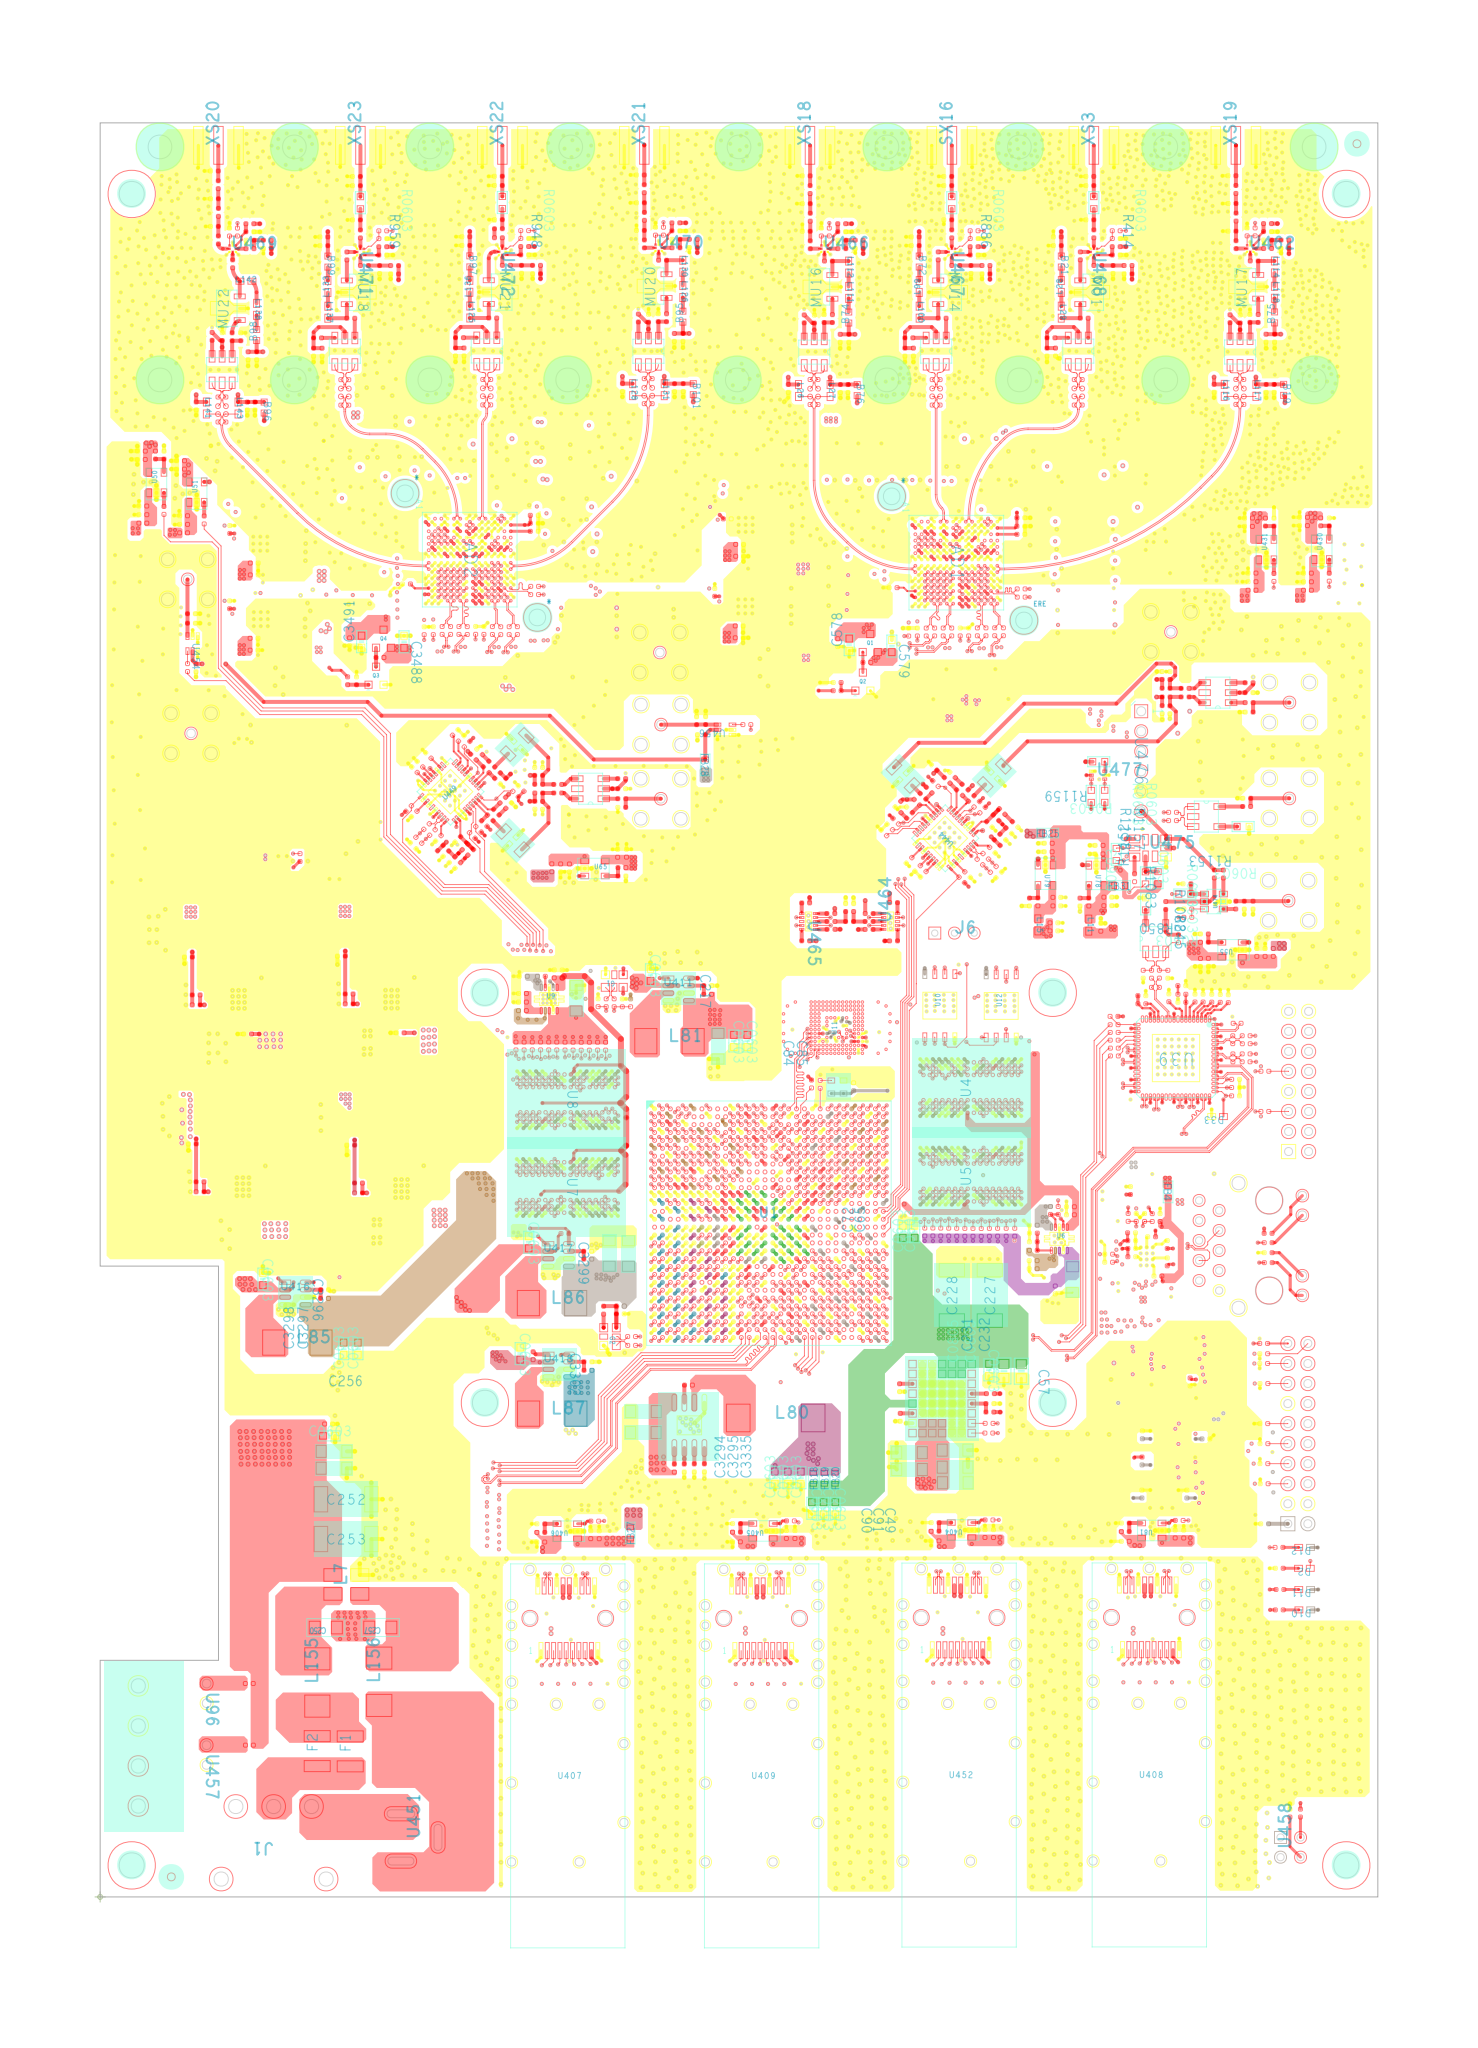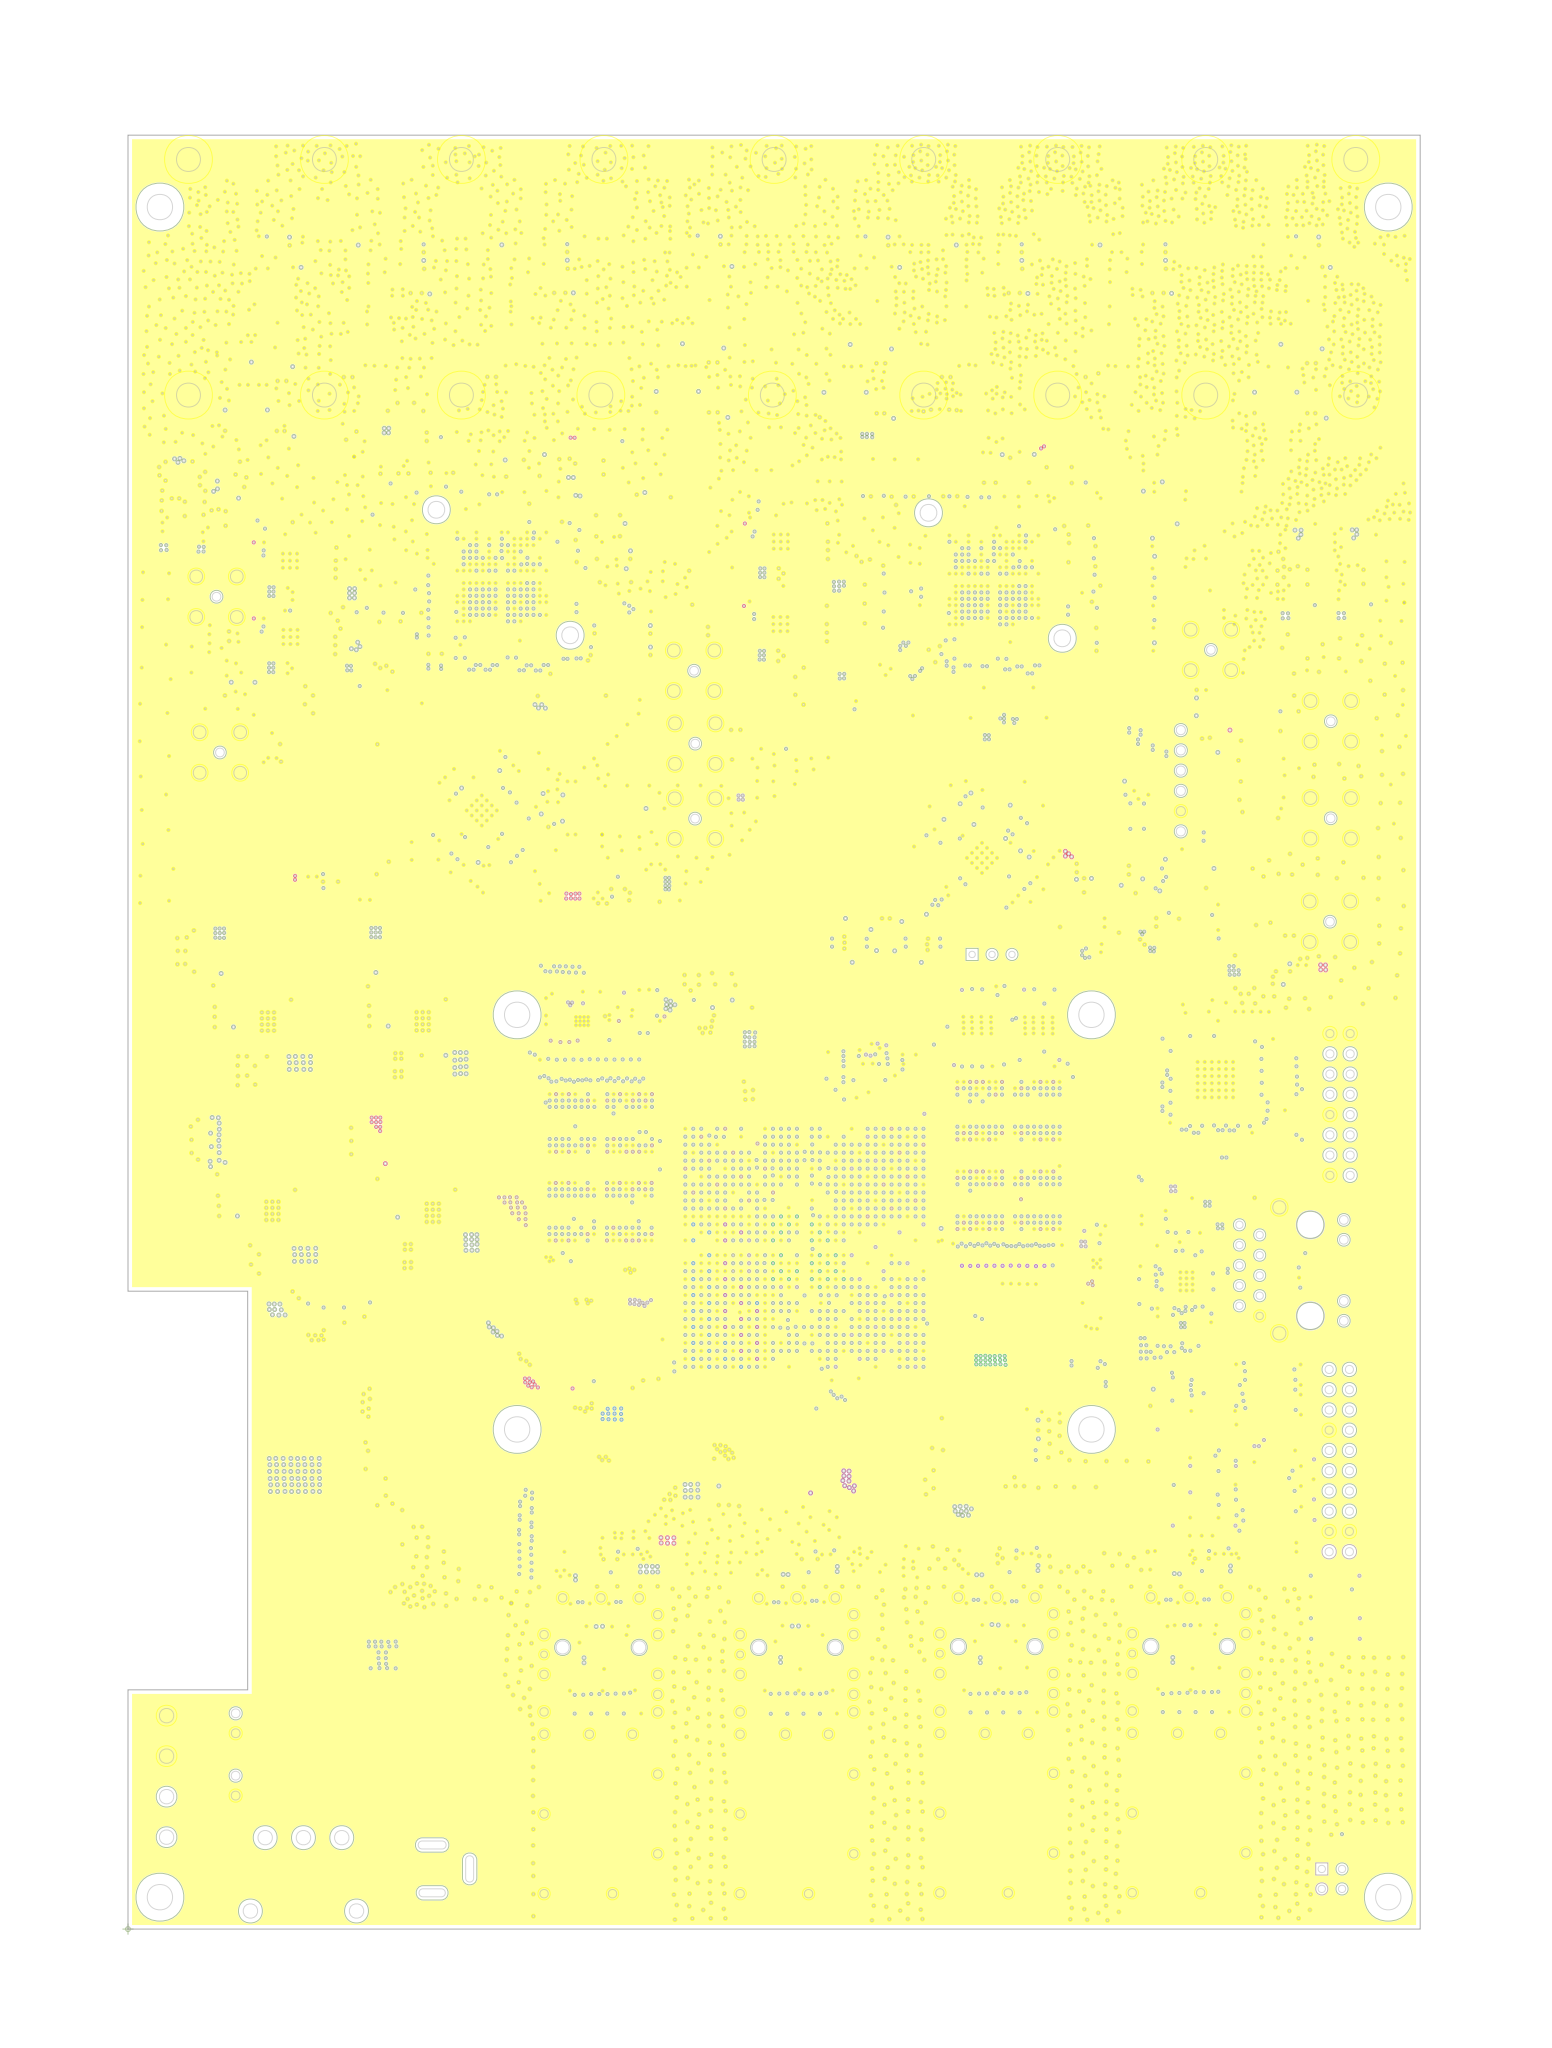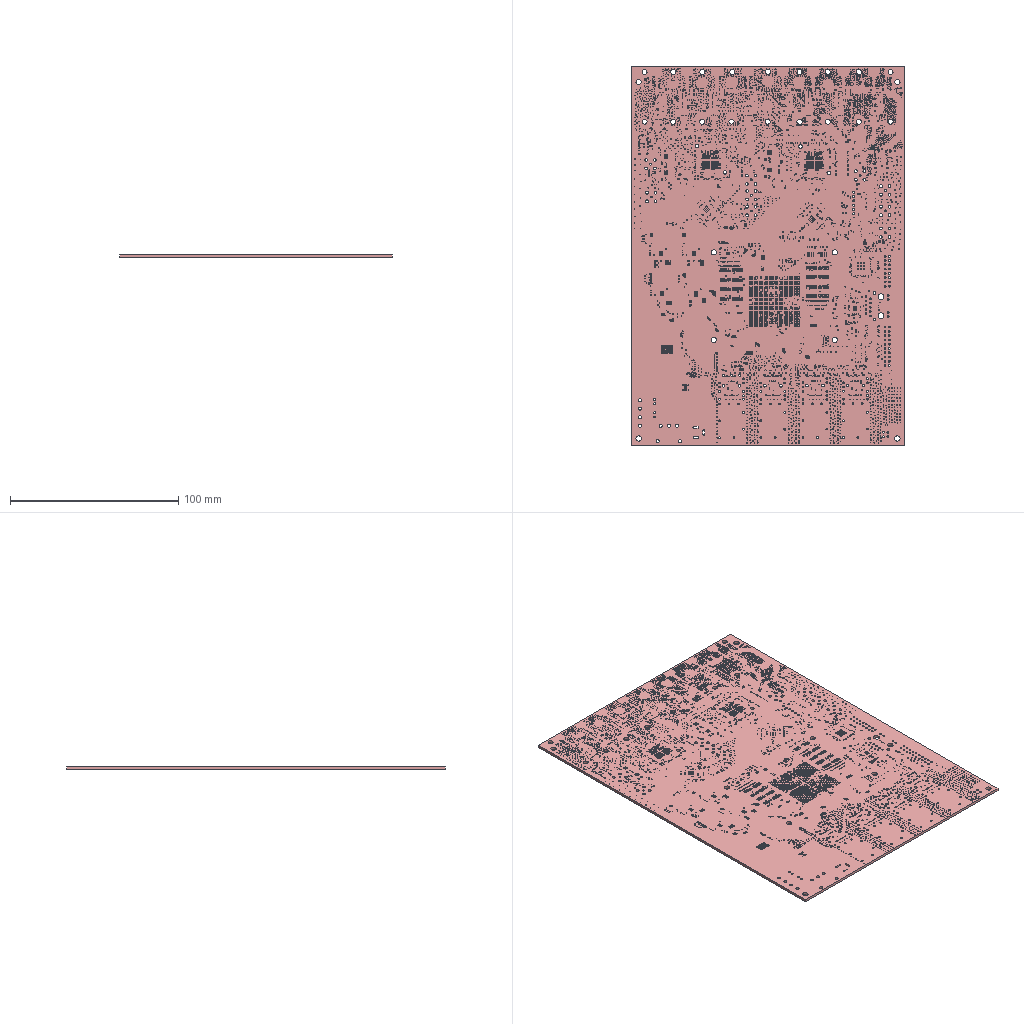Circuit board layout | Cadence Allegro | box 162 x 225 x 1.6 mm
Layer stack:
# Cadence Allegro layer stack of  (unit mm; from the constraint file cross-section; dielectric type: 0 not recorded (Allegro does not mark core vs prepreg), 3 surface material)
index,name,kind,layer,copper_thickness_mm,dielectric_type,dielectric_thickness_mm,dielectric_material,dielectric_constant
0,Top Surface,other,,,,,,
1,TOP,copper,TOP,0.0305,,,,
2,Dielectric1,dielectric,,,0,0.2032,FR-4,4.5
3,GND2,copper,GND2,0.0305,,,,
4,Dielectric2,dielectric,,,0,0.2032,FR-4,4.5
5,SIG3,copper,SIG3,0.0305,,,,
6,Dielectric3,dielectric,,,0,0.2032,FR-4,4.5
7,POWER4,copper,POWER4,0.0305,,,,
8,Dielectric4,dielectric,,,0,0.2032,FR-4,4.5
9,GND5,copper,GND5,0.0305,,,,
10,Dielectric5,dielectric,,,0,0.2032,FR-4,4.5
11,SIG6,copper,SIG6,0.0305,,,,
12,Dielectric6,dielectric,,,0,0.2032,FR-4,4.5
13,POWER7,copper,POWER7,0.0305,,,,
14,Dielectric7,dielectric,,,0,0.2032,FR-4,4.5
15,BOTTOM,copper,BOTTOM,0.0305,,,,
16,Bottom Surface,other,,,,,,
# drill layer pairs: low layer,high layer
drill_pair,TOP,BOTTOM
Part placement, first 543 of 1794 lines:
REFDES,COMP_VALUE,SYM_NAME,SYM_X,SYM_Y,SYM_ROTATE,SYM_MIRROR
25MHZ1,SIT8208AI-2F-33E-25M,3225,5208.251,3540.558,180.000,YES
AD1,AD9371,BGA196,4273.797,6662.298,270.000,NO
AD2,AD9371,BGA196,1844.787,6677.270,270.000,NO
B1,B0603(120R)2A,B0603,4405.607,5888.987,270.000,YES
B2,B0603(120R)2A,B0603,4286.605,5888.999,270.000,YES
B3,B0603(120R)2A,B0603,4053.238,7257.773,90.000,YES
B4,B0603(120R)2A,B0603,3729.200,7257.600,90.000,YES
B5,B0603(120R)2A,B0603,3837.838,7257.117,90.000,YES
B6,B0603(120R)2A,B0603,4156.250,7258.397,90.000,YES
B7,B0603(120R)2A,B0603,3549.608,6505.395,180.000,YES
B8,B0603(120R)2A,B0603,3953.432,7258.123,90.000,YES
B9,B0603(120R)2A,B0603,4976.588,6463.405,0.000,YES
B10,B0603(120R)2A,B0603,3627.097,7257.416,90.000,YES
B11,B0603(120R)2A,B0603,4976.178,6574.105,0.000,YES
B12,B0603(120R)2A,B0603,4975.364,6769.187,0.000,YES
B13,B0603(120R)2A,B0603,3548.000,6409.303,180.000,YES
B14,B0603(120R)2A,B0603,4975.658,6672.293,0.000,YES
B15,B0603(120R)2A,B0603,4973.932,6868.378,0.000,YES
B16,B0603(120R)2A,B0603,3548.890,6693.191,180.000,YES
B17,B0603(120R)2A,B0603,4973.648,6351.366,0.000,YES
B18,B0603(120R)2A,B0603,3549.400,6600.097,180.000,YES
B19,B0603(120R)2A,B0603,5907.800,7552.668,270.000,NO
B21,B0603(120R)2A,B0603,4798.017,8193.507,270.000,NO
B72,B0603(120R)2A,B0603,4088.717,8193.407,270.000,NO
B73,B0603(120R)2A,B0603,5104.886,7024.718,90.000,YES
B74,B0603(120R)2A,B0603,3736.793,7858.695,90.000,NO
B75,B0603(120R)2A,B0603,5862.293,7859.295,90.000,NO
B76,B0603(120R)2A,B0603,3778.842,7551.451,270.000,NO
B77,B0603(120R)2A,B0603,2406.400,6690.500,0.000,YES
B78,B0603(120R)2A,B0603,1100.305,6352.178,270.000,YES
B79,B0603(120R)2A,B0603,2150.138,6006.840,270.000,YES
B80,B0603(120R)2A,B0603,2231.480,6007.048,270.000,YES
B81,B0603(120R)2A,B0603,1283.700,6346.000,270.000,YES
B82,B0603(120R)2A,B0603,2181.100,7127.500,90.000,YES
B83,B0603(120R)2A,B0603,1533.468,7278.589,90.000,YES
B84,B0603(120R)2A,B0603,1178.300,6345.600,270.000,YES
B85,B0603(120R)2A,B0603,1386.571,6345.910,270.000,YES
B86,B0603(120R)2A,B0603,2401.100,6805.800,0.000,YES
B87,B0603(120R)2A,B0603,1644.374,7278.607,90.000,YES
B88,B0603(120R)2A,B0603,1206.300,7281.300,90.000,YES
B89,B0603(120R)2A,B0603,1488.743,7444.574,180.000,YES
B90,B0603(120R)2A,B0603,2400.700,6916.800,0.000,YES
B91,B0603(120R)2A,B0603,1295.385,7280.764,90.000,YES
B92,B0603(120R)2A,B0603,1424.368,7281.109,90.000,YES
B93,B0603(120R)2A,B0603,2476.246,6330.290,0.000,YES
B94,B0603(120R)2A,B0603,2477.386,6437.099,0.000,YES
B95,B0603(120R)2A,B0603,2908.893,7862.995,90.000,NO
B96,B0603(120R)2A,B0603,818.800,7464.268,270.000,NO
B97,B0603(120R)2A,B0603,1845.317,8194.207,270.000,NO
B98,B0603(120R)2A,B0603,781.093,7771.395,90.000,NO
B99,B0603(120R)2A,B0603,1136.817,8193.107,270.000,NO
B100,B0603(120R)2A,B0603,2550.897,6957.122,90.000,YES
B101,B0603(120R)2A,B0603,2960.742,7556.351,270.000,NO
C1,22uF/16V,C0603,3830.654,3338.762,0.000,YES
C2,0.47uF,C0402,3282.110,3399.885,270.000,YES
C3,0.1uF,C0402,3319.624,3399.885,270.000,YES
C4,100uF/6.3V,1206,2541.152,3213.020,90.000,NO
C5,0.47uF,C0402,3552.930,3352.808,180.000,YES
C6,4.7uF,C0402,3672.856,2970.154,270.000,YES
C7,0.1uF,C0402,3761.203,4045.350,270.000,NO
C8,22uF/16V,C0603,3593.157,3287.950,180.000,YES
C9,4.7uF,C0402,3165.053,3246.958,90.000,YES
C10,0.47uF,C0402,3163.712,3129.783,270.000,YES
C11,0.01uF,C0402,3496.001,3698.018,0.000,YES
C13,100uF/6.3V,1206,3084.090,4247.774,270.000,NO
C14,4.7uF,C0402,3434.721,2932.735,90.000,YES
C15,100uF/6.3V,1206,2637.229,3212.797,90.000,NO
C16,4.7uF,C0402,3662.263,3208.192,0.000,YES
C17,100uF/6.3V,1206,3998.258,3294.295,180.000,YES
C18,4.7uF,C0402,3457.064,3151.027,180.000,YES
C19,22uF/16V,C0603,3857.096,2732.465,0.000,YES
C20,4.7uF,C0402,3204.304,3130.532,270.000,YES
C21,22uF/16V,C0603,3712.710,3338.714,180.000,YES
C22,4.7uF,C0402,3028.701,3310.203,180.000,YES
C23,47uF/6.3V,C0603,4255.087,3640.246,0.000,YES
C24,4.7uF,C0402,2989.202,3932.223,0.000,YES
C25,0.47uF,C0402,2948.688,3855.397,180.000,YES
C26,0.01uF,C0402,2830.121,3895.228,0.000,YES
C27,47uF/6.3V,C0603,2643.043,3404.908,90.000,YES
C28,4.7uF,C0402,3202.685,3676.385,90.000,YES
C29,0.47uF,C0402,2191.798,4156.921,0.000,YES
C30,0.01uF,C0402,3085.530,3674.468,90.000,YES
C31,22uF/16V,C0603,3343.337,3904.685,90.000,YES
C32,4.7uF,C0402,3263.279,3695.778,180.000,YES
C33,0.47uF,C0402,3279.240,3836.426,90.000,YES
C34,22uF/16V,C0603,3265.198,3618.237,90.000,YES
C35,4.7uF,C0402,2868.948,3695.869,180.000,YES
C36,0.47uF,C0402,2135.492,3808.029,0.000,YES
C37,22uF/16V,C0603,2274.439,4014.844,180.000,YES
C38,4.7uF,C0402,3790.230,3596.228,90.000,YES
C39,4.7uF,C0402,2828.124,3934.694,0.000,YES
C40,0.47uF,C0402,4571.400,3789.205,90.000,YES
C41,0.47uF,C0402,3086.326,3915.123,180.000,YES
C42,0.47uF,C0402,2098.651,4153.939,180.000,YES
C43,0.47uF,C0402,2989.760,3976.398,0.000,YES
C44,0.47uF,C0402,3163.865,3719.834,270.000,YES
C45,0.47uF,C0402,2337.208,4084.462,270.000,YES
C46,0.01uF,C0402,3593.915,3556.411,90.000,YES
C47,0.01uF,C0402,3692.397,3577.574,0.000,YES
C49,22uF/16V,C0603,3669.926,1940.763,270.000,NO
C50,4.7uF,C0402,3283.598,3284.397,90.000,YES
C51,4.7uF,C0402,3456.957,3269.693,0.000,YES
C52,4.7uF,C0402,3240.206,3286.367,90.000,YES
C53,0.47uF,C0402,3375.202,3152.212,180.000,YES
C54,0.47uF,C0402,3375.775,3191.175,0.000,YES
C55,0.47uF,C0402,3376.301,3233.318,180.000,YES
C56,0.47uF,C0402,3516.162,3212.572,90.000,YES
C57,22uF/16V,C0603,4436.429,2631.932,270.000,NO
C58,4.7uF,C0402,3377.369,3269.745,0.000,YES
C59,4.7uF,C0402,3203.118,3291.095,90.000,YES
C60,4.7uF,C0402,3455.204,3307.943,180.000,YES
C61,0.47uF,C0402,3378.599,3499.208,0.000,YES
C62,0.47uF,C0402,3454.840,3191.970,0.000,YES
C63,0.47uF,C0402,3282.911,3205.983,270.000,YES
C64,0.47uF,C0402,3319.899,3284.661,90.000,YES
C65,22uF/16V,C0603,4066.127,3321.362,90.000,NO
C66,4.7uF,C0402,3375.555,3308.285,180.000,YES
C68,4.7uF,C0402,3164.578,3331.561,270.000,YES
C69,0.47uF,C0402,3240.019,3209.113,270.000,YES
C70,0.47uF,C0402,3243.634,3346.078,0.000,YES
C71,0.47uF,C0402,3203.221,3210.589,90.000,YES
C72,22uF/16V,C0603,4006.967,3320.968,90.000,NO
C73,4.7uF,C0402,3324.988,3520.620,270.000,YES
C74,4.7uF,C0402,3298.114,3463.355,0.000,YES
C75,4.7uF,C0402,3455.381,3379.091,0.000,YES
C76,0.47uF,C0402,3319.238,3205.510,90.000,YES
C77,0.47uF,C0402,3456.495,3231.055,180.000,YES
C78,0.47uF,C0402,3455.189,3345.503,0.000,YES
C79,0.47uF,C0402,3180.481,3461.948,180.000,YES
C80,4.7uF,C0402,3397.536,3400.117,270.000,YES
C81,4.7uF,C0402,3376.975,3464.247,0.000,YES
C82,0.47uF,C0402,3204.432,3400.226,270.000,YES
C83,22uF/16V,C0603,3596.108,3400.652,180.000,YES
C84,22uF/16V,C0603,3163.245,4274.157,270.000,NO
C85,22uF/16V,C0603,3229.807,4273.998,270.000,NO
C86,0.47uF,C0402,3457.062,3498.105,0.000,YES
C87,10uF/10V,C0402,3456.367,3462.528,0.000,YES
C88,22uF/16V,C0603,3329.971,3621.638,270.000,YES
C89,22uF/16V,C0603,3417.758,3592.051,270.000,YES
C90,22uF/16V,C0603,3552.655,1940.553,270.000,NO
C91,22uF/16V,C0603,3611.308,1940.553,270.000,NO
C94,4.7uF,C0402,2947.900,2954.838,0.000,YES
C95,4.7uF,C0402,3003.855,3442.776,90.000,YES
C96,0.47uF,C0402,2945.464,3462.637,180.000,YES
C97,0.47uF,C0402,2928.668,3205.993,270.000,YES
C98,0.47uF,C0402,2944.326,3067.849,180.000,YES
C99,0.47uF,C0402,2929.729,3286.593,90.000,YES
C100,4.7uF,C0402,2769.759,3440.933,270.000,YES
C101,4.7uF,C0402,2808.916,3400.458,90.000,YES
C102,0.47uF,C0402,2866.890,3344.611,180.000,YES
C103,0.47uF,C0402,2770.842,3288.582,270.000,YES
C104,0.47uF,C0402,2770.346,3208.484,270.000,YES
C105,0.47uF,C0402,2866.150,3265.631,180.000,YES
C107,4.7uF,C0402,2957.003,3359.219,180.000,YES
C108,0.47uF,C0402,3025.398,3268.001,0.000,YES
C109,0.01uF,C0402,4452.964,3603.929,0.000,YES
C110,0.01uF,C0402,4452.910,3645.066,180.000,YES
C111,0.01uF,C0402,4512.400,4218.412,180.000,YES
C112,0.01uF,C0402,4512.326,4257.048,0.000,YES
C114,4.7uF,C0402,4157.093,3230.017,270.000,YES
C115,4.7uF,C0402,4116.148,3230.147,270.000,YES
C116,4.7uF,C0402,4276.477,3230.017,270.000,YES
C117,1uF,C0402,4195.753,3229.753,270.000,YES
C118,1uF,C0402,4316.713,3230.017,270.000,YES
C119,1uF,C0402,4236.399,3229.753,270.000,YES
C120,1uF,C0402,4356.965,3230.017,270.000,YES
C121,0.1uF,C0402,4398.458,3230.147,270.000,YES
C122,0.1uF,C0402,4438.840,3230.079,270.000,YES
C123,0.1uF,C0402,4523.188,3230.016,270.000,YES
C124,0.1uF,C0402,4481.455,3230.146,270.000,YES
C125,4.7uF,C0402,4308.410,3768.213,180.000,YES
C132,0.1uF,C0402,4060.502,3489.044,90.000,YES
C133,0.1uF,C0402,4219.623,3769.040,0.000,YES
C134,0.1uF,C0402,4496.172,3791.569,90.000,YES
C135,0.1uF,C0402,4129.276,3768.560,180.000,YES
C136,0.1uF,C0402,4219.313,3549.633,0.000,YES
C137,4.7uF,C0402,4137.020,4211.808,180.000,YES
C138,0.1uF,C0402,4482.343,3865.702,180.000,YES
C139,0.1uF,C0402,4321.272,4214.028,180.000,YES
C140,0.1uF,C0402,4268.090,3870.491,0.000,YES
C141,0.1uF,C0402,4229.989,4213.107,0.000,YES
C142,0.1uF,C0402,4064.019,4138.470,90.000,YES
C143,0.01uF,C0402,4658.410,3314.351,0.000,NO
C144,4.7uF,C0402,4657.886,3353.910,0.000,NO
C145,0.1uF,C0402,4843.347,3406.119,0.000,NO
C146,100uF/6.3V,1206,4854.765,3082.881,270.000,NO
C147,10uF/10V,C0402,4657.323,3136.541,0.000,NO
C148,10uF/10V,C0402,4657.323,3177.093,0.000,NO
C149,10uF/10V,C0402,4767.768,3030.771,90.000,NO
C150,4.7uF,C0402,4782.105,3427.837,90.000,YES
C151,4.7uF,C0402,4843.347,3446.135,0.000,NO
C152,4.7uF,C0402,2370.016,3373.031,0.000,YES
C153,0.1uF,C0402,2574.421,3709.999,180.000,YES
C154,0.1uF,C0402,2398.043,3709.023,180.000,YES
C155,0.1uF,C0402,2486.232,3709.905,180.000,YES
C156,0.1uF,C0402,2458.803,3372.204,180.000,YES
C157,0.1uF,C0402,2559.985,4151.524,180.000,YES
C158,4.7uF,C0402,2549.280,3808.934,0.000,YES
C159,0.1uF,C0402,2467.465,4149.855,180.000,YES
C160,0.1uF,C0402,2554.213,4029.986,180.000,YES
C161,0.1uF,C0402,2549.150,3372.684,0.000,YES
C162,0.1uF,C0402,2456.312,3807.634,180.000,YES
C163,0.1uF,C0402,2365.028,3806.713,0.000,YES
C164,4.7uF,C0402,2359.807,4336.390,90.000,YES
C165,4.7uF,C0402,2074.127,4336.260,90.000,YES
C166,4.7uF,C0402,2481.948,4336.390,90.000,YES
C167,1uF,C0402,2278.925,4335.996,90.000,YES
C168,1uF,C0402,2441.712,4336.654,90.000,YES
C169,1uF,C0402,2319.177,4336.390,90.000,YES
C170,1uF,C0402,2401.066,4336.654,90.000,YES
C171,0.1uF,C0402,2115.461,4335.997,90.000,YES
C172,0.1uF,C0402,2157.192,4335.473,90.000,YES
C173,0.1uF,C0402,2198.625,4335.540,90.000,YES
C174,0.1uF,C0402,2238.614,4335.867,90.000,YES
C175,0.01uF,C0402,2238.134,3487.898,180.000,YES
C176,0.01uF,C0402,2187.696,3935.500,0.000,YES
C177,0.01uF,C0402,2317.112,3684.265,180.000,YES
C178,0.01uF,C0402,2380.424,4148.526,0.000,YES
C179,4.7uF,C0402,2112.164,4597.106,0.000,NO
C180,0.01uF,C0402,2108.013,4511.201,0.000,NO
C181,100uF/6.3V,1206,2376.054,4487.863,90.000,NO
C182,10uF/10V,C0402,2375.648,4445.049,90.000,YES
C183,10uF/10V,C0402,2202.599,4425.134,180.000,YES
C184,10uF/10V,C0402,2293.544,4425.134,0.000,YES
C185,4.7uF,C0402,2281.040,4541.705,0.000,YES
C186,0.1uF,C0402,2306.663,4608.586,270.000,NO
C187,4.7uF,C0402,2266.661,4608.980,270.000,NO
C188,0.1uF,C0402,4137.075,4606.477,0.000,YES
C189,0.1uF,C0402,4442.457,4606.083,0.000,YES
C190,10uF/10V,C0402,3680.505,4151.682,270.000,YES
C191,1uF,C0402,3595.721,4149.056,270.000,YES
C192,0.1uF,C0402,3667.390,4295.548,0.000,YES
C193,10uF/10V,C0402,3798.285,4351.080,0.000,YES
C194,0.1uF,C0402,3780.110,4289.215,270.000,YES
C195,0.1uF,C0402,3666.997,4246.036,0.000,YES
C196,10uF/10V,C0402,3869.359,4242.142,0.000,YES
C197,0.1uF,C0402,3868.835,4292.493,0.000,YES
C198,0.1uF,C0402,3588.556,4291.839,270.000,YES
C199,0.1uF,C0402,3868.835,4198.099,0.000,YES
C200,0.1uF,C0402,2489.044,4580.813,270.000,YES
C201,4.7uF,C0402,2448.178,4580.813,270.000,YES
C202,0.1uF,C0402,2572.059,4580.345,90.000,YES
C203,0.1uF,C0402,2565.664,4464.674,90.000,NO
C204,0.1uF,C0402,2525.900,4464.804,90.000,NO
C205,0.1uF,C0402,2596.400,2911.400,180.000,NO
C206,0.1uF,C0402,3908.531,3207.189,90.000,YES
C207,4.7uF,C0402,3770.989,3233.304,0.000,YES
C208,0.1uF,C0402,2652.855,2797.985,180.000,NO
C209,0.1uF,C0402,2653.119,2753.889,180.000,NO
C210,0.1uF,C0402,3369.153,2103.770,270.000,YES
C211,150pF,C0402,2965.825,2142.235,90.000,YES
C212,2.2uF,C0402,2965.683,2142.131,90.000,NO
C213,10nF,C0402,3016.162,2142.458,90.000,NO
C214,22uF/25V,1206,2711.969,2423.426,0.000,NO
C217,22uF/10V,C0603,2747.145,4604.273,270.000,NO
C219,22uF,C0603,3160.760,4285.788,270.000,YES
C220,22uF,C0603,3084.855,4281.854,270.000,YES
C222,22uF/25V,1206,4040.186,2134.004,0.000,NO
C223,22uF/25V,1206,4268.676,2068.106,180.000,NO
C224,22uF/25V,1206,4040.166,2218.238,0.000,NO
C225,22uF/25V,1206,4267.686,2145.845,180.000,NO
C226,22uF/25V,1206,4267.492,2230.949,180.000,NO
C227,470uF,C7343,4441.112,3003.981,90.000,NO
C228,470uF,C7343,4251.594,3004.145,90.000,NO
C229,47uF,C0805,4511.368,2626.963,270.000,YES
C230,47uF,C0805,4598.202,2626.669,270.000,YES
C231,47uF,C0805,4511.408,2626.375,90.000,NO
C232,47uF,C0805,4598.242,2624.899,90.000,NO
C250,1000pF/1KV,C1206,1126.316,1344.967,180.000,NO
C252,100uF/25V,C7343,1228.043,1985.644,0.000,NO
C253,100uF/25V,C7343,1228.043,1787.054,0.000,NO
C254,22uF/25V,1206,1167.429,2224.818,180.000,NO
C255,22uF/25V,1206,1167.203,2140.482,180.000,NO
C256,4.7uF/25V,C0603,1142.948,2302.052,0.000,NO
C257,1000pF/1KV,C1206,1398.311,1345.391,180.000,NO
C258,0.01uF/25V,C0402,1140.200,2361.400,180.000,NO
C259,1000pF/1KV,C1206,1397.614,1344.475,180.000,YES
C352,100pF,C0402,712.695,5809.871,0.000,YES
C355,1nF,C0402,1380.447,5303.903,0.000,YES
C356,10uF,C0402,1380.321,5343.891,180.000,YES
C365,22uF,C0603,5220.442,1234.619,180.000,YES
C366,0.1uF,C0402,5272.193,1535.570,0.000,YES
C367,22uF,C0603,5300.955,1457.558,180.000,YES
C368,0.1uF,C0402,5185.513,1535.964,180.000,YES
C380,100nF,C0402,5248.691,3296.316,180.000,NO
C381,100nF,C0402,5326.829,3257.485,90.000,NO
C382,100nF,C0402,5326.829,3170.988,90.000,NO
C383,100nF,C0402,5035.416,3374.722,180.000,YES
C384,2.2uF,C0402,5050.675,3480.546,180.000,YES
C385,100nF,C0402,5050.171,3522.732,0.000,YES
C386,4.7uF,C0402,5149.757,3196.646,180.000,NO
C387,100nF,C0402,5149.648,3237.870,0.000,NO
C388,4.7uF,C0402,5148.404,3315.946,180.000,NO
C389,100nF,C0402,5149.061,3276.876,0.000,NO
C390,100nF,C0402,5290.779,3392.428,90.000,NO
C391,100nF,C0402,5280.112,3100.104,180.000,NO
C392,4.7uF,C0402,5101.730,3047.601,180.000,YES
C393,100nF,C0402,5102.136,3005.842,0.000,YES
C394,100nF,C0402,5505.168,3611.138,0.000,YES
C395,2.2uF,C0402,5303.502,2996.149,0.000,YES
C396,100nF,C0402,5142.921,3527.040,90.000,NO
C397,100nF,C0402,5251.981,3391.948,90.000,YES
C398,0.01uF,C0402,5812.761,1863.074,180.000,NO
C399,10uF,C0402,5812.349,1862.970,0.000,YES
C400,100nF,C0402,5095.861,2583.653,180.000,YES
C401,100nF,C0402,5440.963,2571.317,90.000,NO
C402,1uF,C0402,5627.791,4375.463,90.000,YES
C403,0.01uF,C0402,5175.584,4317.224,270.000,YES
C404,1uF,C0402,4995.073,4841.746,270.000,NO
C405,0.01uF,C0402,5243.352,4363.505,270.000,YES
C410,0.01uF,C0402,5361.158,4364.476,270.000,YES
C414,0.01uF,C0402,5518.485,4383.892,180.000,YES
C418,1uF,C0402,4760.990,4863.912,180.000,NO
C419,0.01uF,C0402,5194.707,4139.989,0.000,YES
C422,0.01uF,C0402,5194.918,4198.301,0.000,YES
C426,0.01uF,C0402,5241.692,4013.250,90.000,YES
C427,1uF,C0402,5399.376,4550.038,0.000,NO
C428,180pF,C0402,5399.770,4467.298,180.000,NO
C430,0.01uF,C0402,5301.974,4013.067,90.000,YES
C432,0.01uF,C0402,5361.074,4013.672,90.000,YES
C434,0.01uF,C0402,5420.174,4013.095,90.000,YES
C435,0.1uF,C0402,5334.794,4489.495,90.000,NO
C436,0.1uF,C0402,5248.494,4607.264,90.000,NO
C437,0.1uF,C0402,5287.500,4607.447,90.000,NO
C439,0.01uF,C0402,5478.880,4013.700,90.000,YES
C440,1nF,C0402,5200.129,4459.635,180.000,NO
C441,470nF,C0402,5199.884,4500.223,0.000,NO
C445,0.1uF,C0402,4421.656,6316.956,270.000,NO
C446,1uF,C0402,4074.985,6823.065,180.000,YES
C447,0.1uF,C0402,4378.999,6316.810,270.000,NO
C448,100uF,1206,4469.629,6019.758,0.000,YES
C449,1uF,C0402,4426.940,6085.104,0.000,YES
C450,1uF,C0402,4398.099,6981.916,90.000,YES
C451,1uF,C0402,3748.918,7147.533,0.000,YES
C452,0.01uF,C0402,3749.346,7103.567,0.000,YES
C453,0.1uF,C0402,4508.732,6317.218,270.000,NO
C454,0.1uF,C0402,4421.968,6317.137,90.000,YES
C455,1uF,C0402,3958.405,6537.435,0.000,NO
C456,0.1uF,C0402,4378.995,6316.772,90.000,YES
C457,0.1uF,C0402,4508.779,6317.293,90.000,YES
C458,1uF,C0402,4597.321,6749.600,0.000,YES
C459,1uF,C0402,3858.064,7151.264,0.000,YES
C460,100uF,1206,4222.981,6024.986,180.000,YES
C461,0.1uF,C0402,4465.240,6317.223,90.000,YES
C462,1uF,C0402,4268.513,6130.064,180.000,YES
C463,0.01uF,C0402,4268.358,6087.164,180.000,YES
C464,0.1uF,C0402,4250.703,6316.251,270.000,NO
C465,0.1uF,C0402,4208.409,6316.256,270.000,NO
C466,0.1uF,C0402,4165.418,6316.201,270.000,NO
C467,0.1uF,C0402,4250.446,6316.092,90.000,YES
C468,0.1uF,C0402,4208.435,6316.426,90.000,YES
C469,1uF,C0402,4277.325,6595.195,90.000,YES
C470,0.01uF,C0402,4277.599,6508.325,270.000,YES
C471,0.1uF,C0402,4165.375,6316.269,90.000,YES
C472,0.1uF,C0402,4123.997,6316.204,90.000,YES
C473,0.01uF,C0402,4426.968,6130.368,0.000,YES
C474,0.1uF,C0402,4465.401,6317.258,270.000,NO
C475,0.01uF,C0402,3857.973,7105.722,0.000,YES
C476,0.1uF,C0402,4123.569,6316.054,270.000,NO
C477,1uF,C0402,4073.654,7110.654,0.000,YES
C478,0.01uF,C0402,4073.294,7152.974,0.000,YES
C479,1uF,C0402,4175.745,7111.336,0.000,YES
C480,0.01uF,C0402,4175.865,7153.262,0.000,YES
C481,1uF,C0402,3663.125,6525.233,90.000,YES
C482,0.01uF,C0402,3703.545,6525.353,90.000,YES
C483,1uF,C0402,3972.901,7151.976,0.000,YES
C484,0.01uF,C0402,3973.217,7109.586,0.000,YES
C485,1uF,C0402,4865.951,6444.874,270.000,YES
C486,0.01uF,C0402,4822.773,6444.853,270.000,YES
C487,0R,C0402,3958.306,6578.946,180.000,YES
C488,1uF,C0402,3647.363,7100.609,0.000,YES
C489,0.01uF,C0402,3647.503,7143.653,0.000,YES
C490,100uF,1206,3691.089,7032.129,0.000,YES
C491,1uF,C0402,4826.117,6554.678,270.000,YES
C492,0.01uF,C0402,4867.661,6554.932,270.000,YES
C493,0R,C0402,3958.349,6619.526,180.000,YES
C494,1uF,C0402,4865.757,6748.812,270.000,YES
C495,0.01uF,C0402,4823.761,6748.918,270.000,YES
C496,1uF,C0402,3664.289,6428.545,90.000,YES
C497,0.01uF,C0402,3707.073,6428.340,90.000,YES
C498,1uF,C0402,4822.835,6653.437,270.000,YES
C499,0.01uF,C0402,4865.943,6652.826,270.000,YES
C500,10uF,C0402,5028.049,6848.314,270.000,YES
C501,1uF,C0402,4864.753,6849.005,270.000,YES
C502,0.01uF,C0402,4821.459,6848.913,270.000,YES
C503,1uF,C0402,4595.839,6886.418,180.000,NO
C504,1uF,C0402,4595.748,6844.124,180.000,NO
C505,1uF,C0402,3703.093,6713.232,90.000,YES
C506,0.01uF,C0402,3661.561,6713.561,90.000,YES
C507,10uF,C0402,5028.431,6331.915,270.000,YES
C508,0.01uF,C0402,4821.353,6331.673,270.000,YES
C509,1uF,C0402,4864.739,6332.039,270.000,YES
C510,1uF,C0402,3660.747,6619.490,90.000,YES
C511,0.01uF,C0402,3704.713,6619.468,90.000,YES
C512,10uF,C0402,5030.549,6653.290,270.000,YES
C513,10uF,C0402,5027.481,6750.226,270.000,YES
C514,0.01uF,C0402,3576.759,6750.937,0.000,YES
C515,0.01uF,C0402,5030.025,6444.502,270.000,YES
C516,0.01uF,C0402,5030.731,6554.639,270.000,YES
C517,100uF,1206,3963.741,7399.616,90.000,YES
C518,100uF,1206,4053.967,7399.910,90.000,YES
C519,100uF,1206,3398.062,6094.923,180.000,YES
C520,100uF,1206,3398.950,6183.179,180.000,YES
C536,10uF/10V,C0402,5859.872,7532.525,270.000,NO
C537,0.01uF,C0402,5820.636,7532.557,270.000,NO
C538,0.2pF,C0402,3563.626,7451.933,0.000,NO
C539,NC,C0402,3563.583,7576.701,0.000,NO
C540,3pF,C0402,3565.303,7878.416,270.000,NO
C541,43pF,C0402,3565.477,7878.532,270.000,YES
C542,0.01uF,C0402,5560.478,7532.958,270.000,NO
C545,100pF,C0402,4462.885,6982.332,90.000,YES
C546,100pF,C0402,4507.107,6982.543,90.000,YES
C547,NC,C0402,4492.577,7240.028,180.000,YES
C548,NC,C0402,4493.122,7158.656,0.000,YES
C549,100pF,C0402,4306.359,6980.838,90.000,YES
C550,NC,C0402,4334.669,7235.682,180.000,YES
C551,NC,C0402,4334.808,7155.192,0.000,YES
C552,100pF,C0402,4350.881,6981.049,90.000,YES
C563,10uF,C0402,3190.025,6287.518,180.000,YES
C564,1uF,C0402,3189.980,6346.534,180.000,NO
C565,0.1uF,C0402,3190.036,6287.074,180.000,NO
C566,10uF,C0402,3403.362,6443.148,180.000,YES
C567,1uF,C0402,3403.345,6358.548,0.000,YES
C568,0.1uF,C0402,3403.795,6401.748,0.000,YES
C569,1uF,C0402,3067.900,6513.900,270.000,NO
C570,0.01uF,C0402,3253.375,6602.360,180.000,YES
C577,2.2uF,C0402,3951.607,6236.086,90.000,YES
C578,22uF,C0603,3952.003,6245.620,90.000,NO
C579,22uF,C0603,3739.093,6253.088,270.000,NO
C580,2.2uF,C0402,3682.098,6262.853,90.000,NO
C585,10uF/10V,C0402,213.105,6901.866,0.000,NO
C586,0.1uF,C0402,212.988,6945.078,0.000,NO
C587,10uF/10V,C0402,205.681,7219.312,0.000,NO
C588,0.1uF,C0402,205.416,7177.640,0.000,NO
C589,10uF/10V,C0402,416.535,6853.372,0.000,NO
C590,0.1uF,C0402,416.418,6896.584,0.000,NO
C591,10uF/10V,C0402,401.411,7171.018,0.000,NO
C592,0.1uF,C0402,401.146,7129.346,0.000,NO
C593,10uF/10V,C0402,4778.110,8245.468,0.000,NO
C594,0.1uF,C0402,4777.999,8289.140,0.000,NO
C596,220pF,C0402,4892.744,8194.266,270.000,NO
C597,220pF,C0402,4912.362,7883.137,0.000,NO
C598,NC,C0402,4940.419,8374.200,180.000,NO
C622,10uF,C0402,5773.856,4715.958,270.000,NO
C623,0.01uF,C0402,5815.026,4716.051,270.000,NO
C624,10uF,C0402,5531.854,4666.851,90.000,NO
C625,0.01uF,C0402,5492.538,4666.270,90.000,NO
C634,10uF,C0402,2342.467,5138.012,90.000,NO
C635,0.01uF,C0402,2298.697,5138.319,90.000,NO
C636,10uF,C0402,2583.169,5211.019,270.000,NO
C637,0.01uF,C0402,2627.285,5211.500,270.000,NO
C815,4.7uF,C0402,2967.358,3208.973,270.000,YES
C816,4.7uF,C0402,3142.477,3068.295,0.000,YES
C817,0.47uF,C0402,2944.432,3423.159,180.000,YES
C818,0.47uF,C0402,2964.600,3127.776,270.000,YES
C819,0.47uF,C0402,3007.152,3166.055,270.000,YES
C820,0.47uF,C0402,3043.794,3088.892,270.000,YES
C821,4.7uF,C0402,2787.048,2951.147,180.000,YES
C822,4.7uF,C0402,2787.235,3108.812,180.000,YES
C823,0.47uF,C0402,2787.076,2832.159,180.000,YES
C824,0.47uF,C0402,2865.937,2793.153,180.000,YES
C825,0.47uF,C0402,2786.016,3068.559,180.000,YES
C826,0.47uF,C0402,2786.865,2911.353,180.000,YES
C827,4.7uF,C0402,2944.920,2911.353,180.000,YES
C828,4.7uF,C0402,2866.575,2871.953,180.000,YES
C829,0.47uF,C0402,3023.626,2793.547,180.000,YES
C830,0.47uF,C0402,2944.887,2832.947,180.000,YES
C831,0.47uF,C0402,2866.148,2951.541,180.000,YES
C832,0.47uF,C0402,2866.603,3028.765,180.000,YES
C833,4.7uF,C0402,3141.234,2987.919,0.000,YES
C834,4.7uF,C0402,3043.459,3011.263,90.000,YES
C835,0.47uF,C0402,3121.806,2813.153,270.000,YES
C836,0.47uF,C0402,3141.933,2911.877,0.000,YES
C837,0.47uF,C0402,3023.992,2871.559,180.000,YES
C838,0.47uF,C0402,3025.629,2949.965,180.000,YES
C839,0.47uF,C0402,2866.026,3462.559,180.000,YES
C840,0.47uF,C0402,2866.481,3107.959,180.000,YES
C841,0.47uF,C0402,2865.754,3187.547,180.000,YES
C842,0.47uF,C0402,3606.820,2759.325,270.000,YES
C843,0.47uF,C0402,3498.076,2729.442,270.000,YES
C844,0.47uF,C0402,3808.422,3109.001,0.000,YES
C845,0.47uF,C0402,3590.142,2974.284,90.000,YES
C846,0.47uF,C0402,3239.924,3127.758,90.000,YES
C847,0.47uF,C0402,3316.836,2971.602,270.000,YES
C848,0.47uF,C0402,3204.022,2815.319,90.000,YES
C849,0.47uF,C0402,3262.029,2875.893,180.000,YES
C2866,10uF,C0402,4986.025,5208.062,0.000,NO
C2867,0.01uF,C0402,4986.419,5250.614,0.000,NO
C2868,10uF,C0402,5029.961,4992.046,180.000,NO
C2869,0.01uF,C0402,5029.961,4949.494,180.000,NO
C2870,10uF,C0402,4732.295,5218.650,0.000,NO
C2871,0.01uF,C0402,4732.689,5261.202,0.000,NO
C2872,10uF,C0402,4775.653,4991.028,180.000,NO
C2873,0.01uF,C0402,4775.653,4948.476,180.000,NO
C2880,10nF,C0402,4638.917,4967.817,270.000,NO
C2881,10nF,C0402,4890.987,4967.605,270.000,NO
C2882,10uF,C0402,5366.359,1812.158,270.000,NO
C2883,0.1uF,C0402,5408.911,1811.764,270.000,NO
C2884,10uF,C0402,5116.957,1775.516,0.000,NO
C2886,10nF,C0402,5117.351,1866.830,180.000,NO
C3089,10nF,C0402,318.743,7199.302,90.000,NO
C3090,10nF,C0402,518.900,7000.968,90.000,YES
C3127,10nF,C0402,5512.051,4808.399,180.000,NO
C3130,10nF,C0402,2604.574,5097.469,180.000,NO
C3179,100pF,C0402,691.993,5742.341,270.000,YES
C3180,10uF,C0402,733.037,5742.198,270.000,YES
C3183,100nF,C0402,5425.007,5058.810,0.000,NO
C3192,0.1uF,C0402,5210.408,1286.492,0.000,YES
C3193,22uF,C0603,5160.691,1457.952,0.000,YES
C3194,22uF,C0603,4271.022,1232.870,180.000,YES
C3195,4.7uF,C0402,5200.163,2011.685,90.000,NO
C3196,4.7uF,C0402,5202.527,2307.368,90.000,NO
C3197,22uF,C0603,4211.151,1457.164,0.000,YES
C3198,10uF,C0402,4416.819,1814.522,270.000,NO
C3199,0.1uF,C0402,4459.371,1814.128,270.000,NO
C3200,10uF,C0402,4167.417,1777.880,0.000,NO
C3201,10nF,C0402,4167.811,1868.894,180.000,NO
C3202,0.1uF,C0402,4322.653,1534.782,0.000,YES
C3203,22uF,C0603,4351.415,1456.770,180.000,YES
C3204,22uF,C0603,3285.434,1232.191,180.000,YES
C3205,0.1uF,C0402,3274.600,1284.164,0.000,YES
C3206,0.1uF,C0402,3250.185,1531.236,180.000,YES
C3207,22uF,C0603,3225.363,1453.224,0.000,YES
C3208,10uF,C0402,3425.515,1809.794,270.000,NO
C3209,0.1uF,C0402,3468.067,1809.400,270.000,NO
C3210,10uF,C0402,3176.113,1773.152,0.000,NO
C3211,10nF,C0402,3176.507,1864.166,180.000,NO
C3212,0.1uF,C0402,3336.865,1530.842,0.000,YES
C3213,22uF,C0603,3365.627,1452.830,180.000,YES
C3214,22uF,C0603,2316.770,1232.250,180.000,YES
C3215,0.1uF,C0402,2307.316,1284.382,0.000,YES
C3216,0.1uF,C0402,2282.521,1531.236,180.000,YES
C3217,22uF,C0603,2257.699,1453.224,0.000,YES
C3218,10uF,C0402,2448.789,1808.612,270.000,NO
C3219,0.1uF,C0402,2491.341,1808.218,270.000,NO
C3220,10uF,C0402,2199.387,1771.970,0.000,NO
C3221,10nF,C0402,2199.781,1862.984,180.000,NO
C3222,0.1uF,C0402,2369.201,1530.842,0.000,YES
C3223,22uF,C0603,2397.963,1452.830,180.000,YES
C3224,10uF,C0402,931.568,5154.670,90.000,YES
C3225,0.1uF,C0402,889.016,5154.670,90.000,YES
C3226,10uF,C0402,1166.828,5102.436,270.000,YES
Pad and via stacks, first 105 of 182 lines:
# Allegro (Cadence) via spans and padstacks; design units: ("mils" 3 1000)
# via spans: padstack,start_layer,end_layer,net_example,count
VIA12X20,ETCH/TOP,ETCH/BOTTOM,GND,1619
VIA8_16,ETCH/TOP,ETCH/BOTTOM,GND,5625
# Allegro padstack definitions: name,start_layer,end_layer,drill,plating,holeType,type
SMD_R551X500P0S40,"ETCH/TOP","ETCH/TOP",0.0,"PLATED","none","smd"
2020B,"ETCH/TOP","ETCH/TOP",0.0,"PLATED","none","smd"
R127X152,"ETCH/TOP","ETCH/TOP",0.0,"NON_PLATED","none","smd"
SQ47,"ETCH/TOP","ETCH/TOP",0.0,"NON_PLATED","none","smd"
R41_34X39_37,"ETCH/TOP","ETCH/TOP",0.0,"PLATED","none","smd"
R25_59X39_37,"ETCH/TOP","ETCH/TOP",0.0,"PLATED","none","smd"
R9_84X70_87,"ETCH/TOP","ETCH/TOP",0.0,"PLATED","none","smd"
R29_53X70_87,"ETCH/TOP","ETCH/TOP",0.0,"PLATED","none","smd"
C20,"ETCH/TOP","ETCH/TOP",0.0,"NON_PLATED","none","smd"
RE43_31X19_68,"ETCH/TOP","ETCH/TOP",0.0,"PLATED","none","smd"
RE134X170,"ETCH/TOP","ETCH/TOP",0.0,"PLATED","none","smd"
C12_6,"ETCH/TOP","ETCH/TOP",0.0,"PLATED","none","smd"
O25_59X9_84,"ETCH/TOP","ETCH/TOP",0.0,"PLATED","none","smd"
O9_84X25_59,"ETCH/TOP","ETCH/TOP",0.0,"PLATED","none","smd"
R370_08X144_68-S,"ETCH/TOP","ETCH/TOP",0.0,"PLATED","none","smd"
R324_8X51_18-S,"ETCH/TOP","ETCH/TOP",0.0,"PLATED","none","smd"
S98_42,"ETCH/TOP","ETCH/TOP",0.0,"PLATED","none","smd"
SHAPE9_4X2_4-S,"ETCH/TOP","ETCH/TOP",0.0,"PLATED","none","smd"
R43_31X74_8,"ETCH/TOP","ETCH/TOP",0.0,"PLATED","none","smd"
R19_68X15_75,"ETCH/TOP","ETCH/TOP",0.0,"PLATED","none","smd"
RE39_37X27_56,"ETCH/TOP","ETCH/TOP",0.0,"NON_PLATED","none","smd"
R85X65,"ETCH/TOP","ETCH/TOP",0.0,"PLATED","none","smd"
O13_78X39_37,"ETCH/TOP","ETCH/TOP",0.0,"PLATED","none","smd"
O39_37X13_78,"ETCH/TOP","ETCH/TOP",0.0,"PLATED","none","smd"
S124_02,"ETCH/TOP","ETCH/TOP",0.0,"PLATED","none","smd"
O23_62X9_84,"ETCH/TOP","ETCH/TOP",0.0,"PLATED","none","smd"
O9_84X23_62,"ETCH/TOP","ETCH/TOP",0.0,"PLATED","none","smd"
SHAPE64_22X145_28-S,"ETCH/TOP","ETCH/TOP",0.0,"PLATED","none","smd"
R27_56X190_75-S,"ETCH/TOP","ETCH/TOP",0.0,"PLATED","none","smd"
RE12X30,"ETCH/TOP","ETCH/TOP",0.0,"PLATED","none","smd"
SMD0_45R,"ETCH/TOP","ETCH/TOP",0.0,"PLATED","none","smd"
OB11_03X33_47,"ETCH/TOP","ETCH/TOP",0.0,"PLATED","none","smd"
RE11,"ETCH/TOP","ETCH/TOP",0.0,"PLATED","none","smd"
S15,"ETCH/TOP","ETCH/TOP",0.0,"PLATED","none","smd"
12X35,"ETCH/TOP","ETCH/TOP",0.0,"PLATED","none","smd"
8X35,"ETCH/TOP","ETCH/TOP",0.0,"PLATED","none","smd"
16X83,"ETCH/TOP","ETCH/TOP",0.0,"PLATED","none","smd"
125X300,"ETCH/TOP","ETCH/TOP",0.0,"PLATED","none","smd"
SMD_R98X276P0S30,"ETCH/TOP","ETCH/TOP",0.0,"PLATED","none","smd"
SMD_R98X433P0S30,"ETCH/TOP","ETCH/TOP",0.0,"PLATED","none","smd"
SMD_R98X276P0S10,"ETCH/TOP","ETCH/TOP",0.0,"PLATED","none","smd"
SMD_R98X433P0S10,"ETCH/TOP","ETCH/TOP",0.0,"PLATED","none","smd"
SMD_R236X669P0S40,"ETCH/TOP","ETCH/TOP",0.0,"PLATED","none","smd"
SMD_R236X669P0S30,"ETCH/TOP","ETCH/TOP",0.0,"PLATED","none","smd"
SMD_R98X433S30,"ETCH/TOP","ETCH/TOP",0.0,"PLATED","none","smd"
SMD_S50P0S40,"ETCH/TOP","ETCH/TOP",0.0,"PLATED","none","smd"
SMD_R510X80P0S0,"ETCH/TOP","ETCH/TOP",0.0,"PLATED","none","smd"
SMD_R810X100P0S0,"ETCH/TOP","ETCH/TOP",0.0,"PLATED","none","smd"
Y10,"ETCH/TOP","ETCH/TOP",0.0,"NON_PLATED","none","smd"
SMD45_50,"ETCH/TOP","ETCH/TOP",0.0,"PLATED","none","smd"
SMD35_32,"ETCH/TOP","ETCH/TOP",0.0,"PLATED","none","smd"
C31_5D31_5N,"ETCH/TOP","ETCH/BOTTOM",31.5,"PLATED","circle_drill","through"
Y300_1,"ETCH/TOP","ETCH/BOTTOM",125.0,"NON_PLATED","circle_drill","through"
Y31,"ETCH/TOP","ETCH/BOTTOM",62.988,"PLATED","circle_drill","through"
VIA8_16,"ETCH/TOP","ETCH/BOTTOM",8.0,"PLATED","circle_drill","through"
VIA12X20,"ETCH/TOP","ETCH/BOTTOM",12.0,"PLATED","circle_drill","through"
Y3_MARK,"ETCH/TOP","ETCH/TOP",0.0,"PLATED","none","smd"
OB2X5,"ETCH/TOP","ETCH/BOTTOM",39.37,"PLATED","oval slot","through"
SMD_R394X300P0S10,"ETCH/TOP","ETCH/TOP",0.0,"PLATED","none","smd"
C14,"ETCH/TOP","ETCH/TOP",0.0,"PLATED","none","smd"
SMD82X112,"ETCH/TOP","ETCH/TOP",0.0,"PLATED","none","smd"
SMD55_63,"ETCH/TOP","ETCH/TOP",0.0,"PLATED","none","smd"
R12X8,"ETCH/TOP","ETCH/TOP",0.0,"NON_PLATED","none","smd"
RECT24X32,"ETCH/TOP","ETCH/TOP",0.0,"PLATED","none","smd"
Y17,"ETCH/TOP","ETCH/BOTTOM",43.307,"PLATED","circle_drill","through"
SMD40X30,"ETCH/TOP","ETCH/TOP",0.0,"PLATED","none","smd"
RX57Y29D0T,"ETCH/TOP","ETCH/TOP",0.0,"NON_PLATED","none","smd"
SMD_R709X1417P0S10,"ETCH/TOP","ETCH/TOP",0.0,"PLATED","none","smd"
SMD_R340X500P0S10,"ETCH/TOP","ETCH/TOP",0.0,"PLATED","none","smd"
SMD_R340X1000P0S10,"ETCH/TOP","ETCH/TOP",0.0,"PLATED","none","smd"
PSM_091S_PM,"ETCH/TOP","ETCH/TOP",0.0,"NON_PLATED","none","smd"
SMD30_32,"ETCH/TOP","ETCH/TOP",0.0,"PLATED","none","smd"
SMD40_45,"ETCH/TOP","ETCH/TOP",0.0,"PLATED","none","smd"
SMDR1_68X1_88,"ETCH/TOP","ETCH/TOP",0.0,"PLATED","none","smd"
SMDR1_5X0_28,"ETCH/TOP","ETCH/TOP",0.0,"PLATED","none","smd"
OB12X33_SM1X2,"ETCH/TOP","ETCH/TOP",0.0,"PLATED","none","smd"
236X236_SM2X2,"ETCH/TOP","ETCH/TOP",0.0,"PLATED","none","smd"
RCT_0_022X0_055_ROT_90_00_TOP,"ETCH/TOP","ETCH/TOP",0.0,"NON_PLATED","none","smd"
OBL_0_022X0_055_ROT_90_00_TOP,"ETCH/TOP","ETCH/TOP",0.0,"NON_PLATED","none","smd"
RX148Y148D0T,"ETCH/TOP","ETCH/TOP",0.0,"PLATED","none","smd"
RX10Y32D0T,"ETCH/TOP","ETCH/TOP",0.0,"PLATED","none","smd"
SMD_S300P0S10,"ETCH/TOP","ETCH/TOP",0.0,"PLATED","none","smd"
SMD_R787X315P0S40,"ETCH/TOP","ETCH/TOP",0.0,"PLATED","none","smd"
SMD_R571X177P0S40,"ETCH/TOP","ETCH/TOP",0.0,"PLATED","none","smd"
SMD_R1299X551P0S40,"ETCH/TOP","ETCH/TOP",0.0,"PLATED","none","smd"
PTH_O787X1811SLOT472X1457S40,"ETCH/TOP","ETCH/BOTTOM",47.24,"PLATED","oval slot","through"
BGA10_SMD0X619,"ETCH/TOP","ETCH/TOP",0.0,"NON_PLATED","none","smd"
PTH_C610D400S40,"ETCH/TOP","ETCH/BOTTOM",40.0,"PLATED","circle_drill","through"
PTH_C610D480S40,"ETCH/TOP","ETCH/BOTTOM",48.0,"PLATED","circle_drill","through"
PTH_C1016D720S40,"ETCH/TOP","ETCH/BOTTOM",72.0,"PLATED","circle_drill","through"
MEC_C1280D1280_NPS40,"ETCH/TOP","ETCH/BOTTOM",127.949,"NON_PLATED","circle_drill","through"
SMD_R118X315P0S20,"ETCH/TOP","ETCH/TOP",0.0,"PLATED","none","smd"
SMD_O315X118P0S20,"ETCH/TOP","ETCH/TOP",0.0,"PLATED","none","smd"
SMD_S1417P0S20,"ETCH/TOP","ETCH/TOP",0.0,"PLATED","none","smd"
SMD_O428X143P0S20,"ETCH/TOP","ETCH/TOP",0.0,"PLATED","none","smd"
SMD_O143X428P0S20,"ETCH/TOP","ETCH/TOP",0.0,"PLATED","none","smd"
SMD_S1240P0S20,"ETCH/TOP","ETCH/TOP",0.0,"PLATED","none","smd"
S_950X950_1,"ETCH/TOP","ETCH/TOP",0.0,"NON_PLATED","none","smd"
R150X121,"ETCH/TOP","ETCH/TOP",0.0,"NON_PLATED","none","smd"
126X67SMD,"ETCH/TOP","ETCH/TOP",0.0,"PLATED","none","smd"